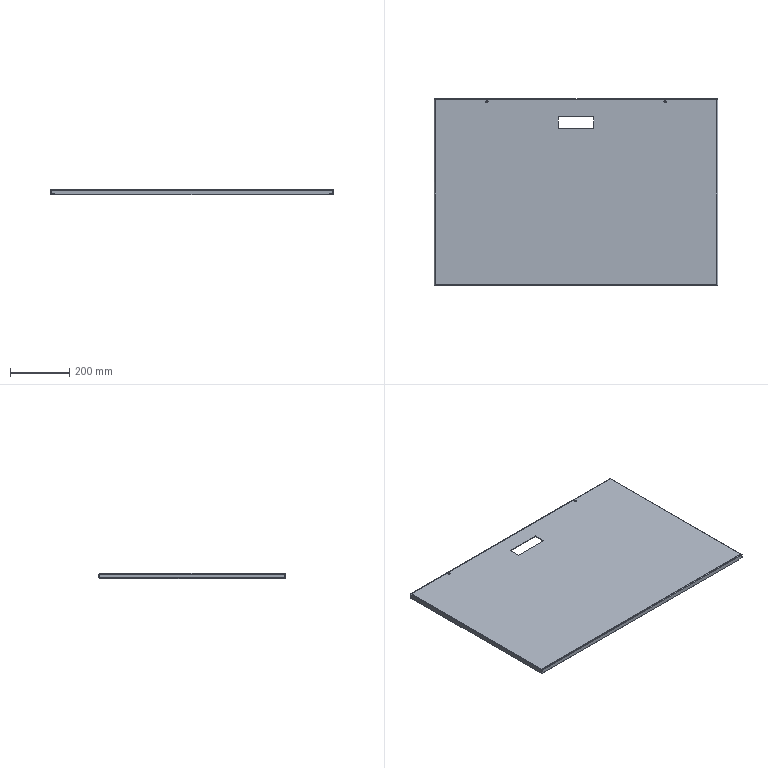Part | STEP file | 400v80 Rear Door Upper | 1 solid | 88 faces | box 955 x 627 x 17 mm | volume 1331439 mm3 | plane 58 | cylinder 22 | spline 8 | commonest cylinder face diameters 7 x8 1 x7 5 x7